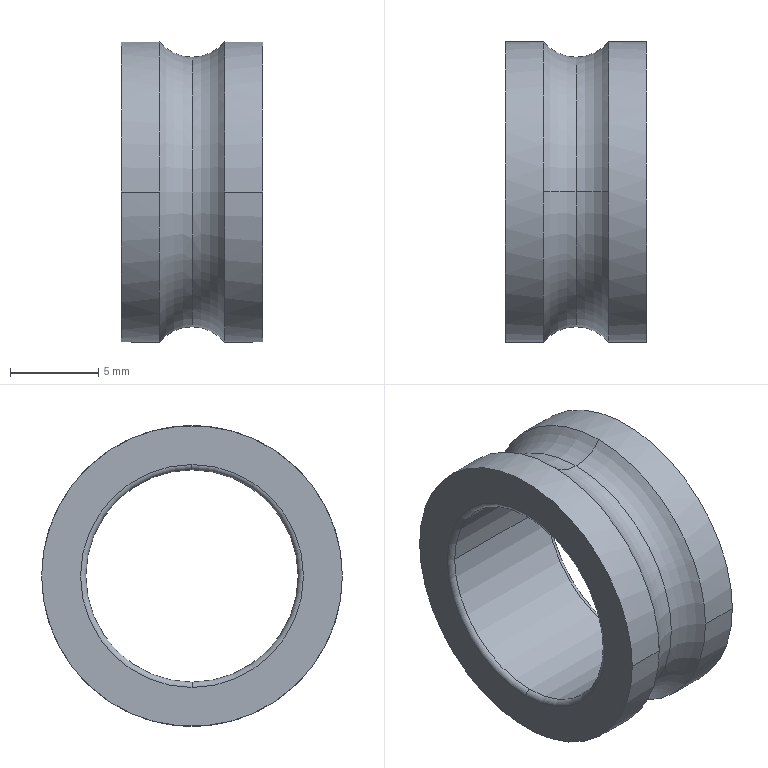Part | STEP file | skf_bearing_6001_2_02 | 1 solid | 16 faces | box 8 x 17 x 17 mm | volume 793.588 mm3 | torus 8 | cylinder 6 | plane 2 | commonest cylinder face diameters 17 x4 12 x2
STEP:
#1=CARTESIAN_POINT('',(5.849,0.,-8.5));
#2=VERTEX_POINT('',#1);
#3=CARTESIAN_POINT('',(4.,0.,-7.619));
#4=VERTEX_POINT('',#3);
#5=CARTESIAN_POINT('',(4.,0.,-10.));
#6=DIRECTION('',(0.,-1.,0.));
#7=DIRECTION('',(0.,0.,-1.));
#8=AXIS2_PLACEMENT_3D('',#5,#6,#7);
#9=CIRCLE('',#8,2.381);
#10=EDGE_CURVE('',#2,#4,#9,.T.);
#11=ORIENTED_EDGE('',*,*,#10,.T.);
#12=CARTESIAN_POINT('',(4.,0.,7.619));
#13=VERTEX_POINT('',#12);
#14=CARTESIAN_POINT('',(4.,0.,0.));
#15=DIRECTION('',(1.,0.,0.));
#16=DIRECTION('',(0.,0.,-1.));
#17=AXIS2_PLACEMENT_3D('',#14,#15,#16);
#18=CIRCLE('',#17,7.619);
#19=EDGE_CURVE('',#4,#13,#18,.T.);
#20=ORIENTED_EDGE('',*,*,#19,.T.);
#21=CARTESIAN_POINT('',(5.849,0.,8.5));
#22=VERTEX_POINT('',#21);
#23=CARTESIAN_POINT('',(4.,0.,10.));
#24=DIRECTION('',(0.,1.,0.));
#25=DIRECTION('',(0.,0.,1.));
#26=AXIS2_PLACEMENT_3D('',#23,#24,#25);
#27=CIRCLE('',#26,2.381);
#28=EDGE_CURVE('',#22,#13,#27,.T.);
#29=ORIENTED_EDGE('',*,*,#28,.F.);
#30=CARTESIAN_POINT('',(5.849,8.5,0.));
#31=VERTEX_POINT('',#30);
#32=CARTESIAN_POINT('',(5.849,0.,0.));
#33=DIRECTION('',(1.,0.,0.));
#34=DIRECTION('',(0.,1.,0.));
#35=AXIS2_PLACEMENT_3D('',#32,#33,#34);
#36=CIRCLE('',#35,8.5);
#37=EDGE_CURVE('',#31,#22,#36,.T.);
#38=ORIENTED_EDGE('',*,*,#37,.F.);
#39=CARTESIAN_POINT('',(5.849,0.,0.));
#40=DIRECTION('',(1.,0.,0.));
#41=DIRECTION('',(0.,1.,0.));
#42=AXIS2_PLACEMENT_3D('',#39,#40,#41);
#43=CIRCLE('',#42,8.5);
#44=EDGE_CURVE('',#2,#31,#43,.T.);
#45=ORIENTED_EDGE('',*,*,#44,.F.);
#46=EDGE_LOOP('',(#11,#20,#29,#38,#45));
#47=FACE_OUTER_BOUND('',#46,.T.);
#48=CARTESIAN_POINT('',(4.,0.,0.));
#49=DIRECTION('',(1.,0.,0.));
#50=DIRECTION('',(0.,0.,-1.));
#51=AXIS2_PLACEMENT_3D('',#48,#49,#50);
#52=TOROIDAL_SURFACE('',#51,10.,2.381);
#53=ADVANCED_FACE('',(#47),#52,.F.);
#54=ORIENTED_EDGE('',*,*,#28,.T.);
#55=CARTESIAN_POINT('',(4.,0.,0.));
#56=DIRECTION('',(1.,0.,0.));
#57=DIRECTION('',(0.,0.,-1.));
#58=AXIS2_PLACEMENT_3D('',#55,#56,#57);
#59=CIRCLE('',#58,7.619);
#60=EDGE_CURVE('',#13,#4,#59,.T.);
#61=ORIENTED_EDGE('',*,*,#60,.T.);
#62=ORIENTED_EDGE('',*,*,#10,.F.);
#63=CARTESIAN_POINT('',(5.849,-8.5,0.));
#64=VERTEX_POINT('',#63);
#65=CARTESIAN_POINT('',(5.849,0.,0.));
#66=DIRECTION('',(1.,0.,0.));
#67=DIRECTION('',(0.,1.,0.));
#68=AXIS2_PLACEMENT_3D('',#65,#66,#67);
#69=CIRCLE('',#68,8.5);
#70=EDGE_CURVE('',#64,#2,#69,.T.);
#71=ORIENTED_EDGE('',*,*,#70,.F.);
#72=CARTESIAN_POINT('',(5.849,0.,0.));
#73=DIRECTION('',(1.,0.,0.));
#74=DIRECTION('',(0.,1.,0.));
#75=AXIS2_PLACEMENT_3D('',#72,#73,#74);
#76=CIRCLE('',#75,8.5);
#77=EDGE_CURVE('',#22,#64,#76,.T.);
#78=ORIENTED_EDGE('',*,*,#77,.F.);
#79=EDGE_LOOP('',(#54,#61,#62,#71,#78));
#80=FACE_OUTER_BOUND('',#79,.T.);
#81=CARTESIAN_POINT('',(4.,0.,0.));
#82=DIRECTION('',(1.,0.,0.));
#83=DIRECTION('',(0.,0.,-1.));
#84=AXIS2_PLACEMENT_3D('',#81,#82,#83);
#85=TOROIDAL_SURFACE('',#84,10.,2.381);
#86=ADVANCED_FACE('',(#80),#85,.F.);
#87=CARTESIAN_POINT('',(8.,0.,-6.3));
#88=VERTEX_POINT('',#87);
#89=CARTESIAN_POINT('',(8.,0.,6.3));
#90=VERTEX_POINT('',#89);
#91=CARTESIAN_POINT('',(8.,0.,0.));
#92=DIRECTION('',(1.,0.,0.));
#93=DIRECTION('',(0.,1.,0.));
#94=AXIS2_PLACEMENT_3D('',#91,#92,#93);
#95=CIRCLE('',#94,6.3);
#96=EDGE_CURVE('',#88,#90,#95,.T.);
#97=ORIENTED_EDGE('',*,*,#96,.T.);
#98=CARTESIAN_POINT('',(7.7,0.,6.));
#99=VERTEX_POINT('',#98);
#100=CARTESIAN_POINT('',(7.7,0.,6.3));
#101=DIRECTION('',(0.,1.,0.));
#102=DIRECTION('',(0.,0.,1.));
#103=AXIS2_PLACEMENT_3D('',#100,#101,#102);
#104=CIRCLE('',#103,0.3);
#105=EDGE_CURVE('',#90,#99,#104,.T.);
#106=ORIENTED_EDGE('',*,*,#105,.T.);
#107=CARTESIAN_POINT('',(7.7,6.,0.));
#108=VERTEX_POINT('',#107);
#109=CARTESIAN_POINT('',(7.7,0.,0.));
#110=DIRECTION('',(1.,0.,0.));
#111=DIRECTION('',(0.,1.,0.));
#112=AXIS2_PLACEMENT_3D('',#109,#110,#111);
#113=CIRCLE('',#112,6.);
#114=EDGE_CURVE('',#108,#99,#113,.T.);
#115=ORIENTED_EDGE('',*,*,#114,.F.);
#116=CARTESIAN_POINT('',(7.7,0.,-6.));
#117=VERTEX_POINT('',#116);
#118=CARTESIAN_POINT('',(7.7,0.,0.));
#119=DIRECTION('',(1.,0.,0.));
#120=DIRECTION('',(0.,1.,0.));
#121=AXIS2_PLACEMENT_3D('',#118,#119,#120);
#122=CIRCLE('',#121,6.);
#123=EDGE_CURVE('',#117,#108,#122,.T.);
#124=ORIENTED_EDGE('',*,*,#123,.F.);
#125=CARTESIAN_POINT('',(7.7,0.,-6.3));
#126=DIRECTION('',(0.,-1.,0.));
#127=DIRECTION('',(0.,0.,-1.));
#128=AXIS2_PLACEMENT_3D('',#125,#126,#127);
#129=CIRCLE('',#128,0.3);
#130=EDGE_CURVE('',#88,#117,#129,.T.);
#131=ORIENTED_EDGE('',*,*,#130,.F.);
#132=EDGE_LOOP('',(#97,#106,#115,#124,#131));
#133=FACE_OUTER_BOUND('',#132,.T.);
#134=CARTESIAN_POINT('',(7.7,0.,0.));
#135=DIRECTION('',(1.,0.,0.));
#136=DIRECTION('',(0.,0.,-1.));
#137=AXIS2_PLACEMENT_3D('',#134,#135,#136);
#138=TOROIDAL_SURFACE('',#137,6.3,0.3);
#139=ADVANCED_FACE('',(#133),#138,.T.);
#140=ORIENTED_EDGE('',*,*,#114,.T.);
#141=CARTESIAN_POINT('',(7.7,-6.,0.));
#142=VERTEX_POINT('',#141);
#143=CARTESIAN_POINT('',(7.7,0.,0.));
#144=DIRECTION('',(1.,0.,0.));
#145=DIRECTION('',(0.,1.,0.));
#146=AXIS2_PLACEMENT_3D('',#143,#144,#145);
#147=CIRCLE('',#146,6.);
#148=EDGE_CURVE('',#99,#142,#147,.T.);
#149=ORIENTED_EDGE('',*,*,#148,.T.);
#150=CARTESIAN_POINT('',(0.3,-6.,0.));
#151=VERTEX_POINT('',#150);
#152=CARTESIAN_POINT('',(4.,-6.,0.));
#153=DIRECTION('',(-1.,0.,0.));
#154=VECTOR('',#153,1000.);
#155=LINE('',#152,#154);
#156=EDGE_CURVE('',#142,#151,#155,.T.);
#157=ORIENTED_EDGE('',*,*,#156,.T.);
#158=CARTESIAN_POINT('',(0.3,0.,6.));
#159=VERTEX_POINT('',#158);
#160=CARTESIAN_POINT('',(0.3,0.,0.));
#161=DIRECTION('',(1.,0.,0.));
#162=DIRECTION('',(0.,1.,0.));
#163=AXIS2_PLACEMENT_3D('',#160,#161,#162);
#164=CIRCLE('',#163,6.);
#165=EDGE_CURVE('',#159,#151,#164,.T.);
#166=ORIENTED_EDGE('',*,*,#165,.F.);
#167=CARTESIAN_POINT('',(0.3,6.,0.));
#168=VERTEX_POINT('',#167);
#169=CARTESIAN_POINT('',(0.3,0.,0.));
#170=DIRECTION('',(1.,0.,0.));
#171=DIRECTION('',(0.,1.,0.));
#172=AXIS2_PLACEMENT_3D('',#169,#170,#171);
#173=CIRCLE('',#172,6.);
#174=EDGE_CURVE('',#168,#159,#173,.T.);
#175=ORIENTED_EDGE('',*,*,#174,.F.);
#176=CARTESIAN_POINT('',(4.,6.,0.));
#177=DIRECTION('',(-1.,0.,0.));
#178=VECTOR('',#177,1000.);
#179=LINE('',#176,#178);
#180=EDGE_CURVE('',#108,#168,#179,.T.);
#181=ORIENTED_EDGE('',*,*,#180,.F.);
#182=EDGE_LOOP('',(#140,#149,#157,#166,#175,#181));
#183=FACE_OUTER_BOUND('',#182,.T.);
#184=CARTESIAN_POINT('',(4.,0.,0.));
#185=DIRECTION('',(-1.,0.,0.));
#186=DIRECTION('',(0.,1.,0.));
#187=AXIS2_PLACEMENT_3D('',#184,#185,#186);
#188=CYLINDRICAL_SURFACE('',#187,6.);
#189=ADVANCED_FACE('',(#183),#188,.F.);
#190=CARTESIAN_POINT('',(0.3,0.,-6.));
#191=VERTEX_POINT('',#190);
#192=CARTESIAN_POINT('',(0.3,0.,0.));
#193=DIRECTION('',(1.,0.,0.));
#194=DIRECTION('',(0.,1.,0.));
#195=AXIS2_PLACEMENT_3D('',#192,#193,#194);
#196=CIRCLE('',#195,6.);
#197=EDGE_CURVE('',#191,#168,#196,.T.);
#198=ORIENTED_EDGE('',*,*,#197,.T.);
#199=ORIENTED_EDGE('',*,*,#174,.T.);
#200=CARTESIAN_POINT('',(0.,0.,6.3));
#201=VERTEX_POINT('',#200);
#202=CARTESIAN_POINT('',(0.3,0.,6.3));
#203=DIRECTION('',(0.,1.,0.));
#204=DIRECTION('',(0.,0.,1.));
#205=AXIS2_PLACEMENT_3D('',#202,#203,#204);
#206=CIRCLE('',#205,0.3);
#207=EDGE_CURVE('',#159,#201,#206,.T.);
#208=ORIENTED_EDGE('',*,*,#207,.T.);
#209=CARTESIAN_POINT('',(0.,0.,-6.3));
#210=VERTEX_POINT('',#209);
#211=CARTESIAN_POINT('',(0.,0.,0.));
#212=DIRECTION('',(1.,0.,0.));
#213=DIRECTION('',(0.,1.,0.));
#214=AXIS2_PLACEMENT_3D('',#211,#212,#213);
#215=CIRCLE('',#214,6.3);
#216=EDGE_CURVE('',#210,#201,#215,.T.);
#217=ORIENTED_EDGE('',*,*,#216,.F.);
#218=CARTESIAN_POINT('',(0.3,0.,-6.3));
#219=DIRECTION('',(0.,-1.,0.));
#220=DIRECTION('',(0.,0.,-1.));
#221=AXIS2_PLACEMENT_3D('',#218,#219,#220);
#222=CIRCLE('',#221,0.3);
#223=EDGE_CURVE('',#191,#210,#222,.T.);
#224=ORIENTED_EDGE('',*,*,#223,.F.);
#225=EDGE_LOOP('',(#198,#199,#208,#217,#224));
#226=FACE_OUTER_BOUND('',#225,.T.);
#227=CARTESIAN_POINT('',(0.3,0.,0.));
#228=DIRECTION('',(1.,0.,0.));
#229=DIRECTION('',(0.,0.,-1.));
#230=AXIS2_PLACEMENT_3D('',#227,#228,#229);
#231=TOROIDAL_SURFACE('',#230,6.3,0.3);
#232=ADVANCED_FACE('',(#226),#231,.T.);
#233=CARTESIAN_POINT('',(2.151,-8.5,0.));
#234=VERTEX_POINT('',#233);
#235=CARTESIAN_POINT('',(2.151,0.,-8.5));
#236=VERTEX_POINT('',#235);
#237=CARTESIAN_POINT('',(2.151,0.,0.));
#238=DIRECTION('',(1.,0.,0.));
#239=DIRECTION('',(0.,1.,0.));
#240=AXIS2_PLACEMENT_3D('',#237,#238,#239);
#241=CIRCLE('',#240,8.5);
#242=EDGE_CURVE('',#234,#236,#241,.T.);
#243=ORIENTED_EDGE('',*,*,#242,.F.);
#244=CARTESIAN_POINT('',(0.,-8.5,0.));
#245=VERTEX_POINT('',#244);
#246=CARTESIAN_POINT('',(1.075,-8.5,0.));
#247=DIRECTION('',(-1.,0.,0.));
#248=VECTOR('',#247,1000.);
#249=LINE('',#246,#248);
#250=EDGE_CURVE('',#234,#245,#249,.T.);
#251=ORIENTED_EDGE('',*,*,#250,.T.);
#252=CARTESIAN_POINT('',(0.,8.5,0.));
#253=VERTEX_POINT('',#252);
#254=CARTESIAN_POINT('',(0.,0.,0.));
#255=DIRECTION('',(1.,0.,0.));
#256=DIRECTION('',(0.,1.,0.));
#257=AXIS2_PLACEMENT_3D('',#254,#255,#256);
#258=CIRCLE('',#257,8.5);
#259=EDGE_CURVE('',#245,#253,#258,.T.);
#260=ORIENTED_EDGE('',*,*,#259,.T.);
#261=CARTESIAN_POINT('',(2.151,8.5,0.));
#262=VERTEX_POINT('',#261);
#263=CARTESIAN_POINT('',(1.075,8.5,0.));
#264=DIRECTION('',(-1.,0.,0.));
#265=VECTOR('',#264,1000.);
#266=LINE('',#263,#265);
#267=EDGE_CURVE('',#262,#253,#266,.T.);
#268=ORIENTED_EDGE('',*,*,#267,.F.);
#269=CARTESIAN_POINT('',(2.151,0.,0.));
#270=DIRECTION('',(1.,0.,0.));
#271=DIRECTION('',(0.,1.,0.));
#272=AXIS2_PLACEMENT_3D('',#269,#270,#271);
#273=CIRCLE('',#272,8.5);
#274=EDGE_CURVE('',#236,#262,#273,.T.);
#275=ORIENTED_EDGE('',*,*,#274,.F.);
#276=EDGE_LOOP('',(#243,#251,#260,#268,#275));
#277=FACE_OUTER_BOUND('',#276,.T.);
#278=CARTESIAN_POINT('',(1.075,0.,0.));
#279=DIRECTION('',(-1.,0.,0.));
#280=DIRECTION('',(0.,1.,0.));
#281=AXIS2_PLACEMENT_3D('',#278,#279,#280);
#282=CYLINDRICAL_SURFACE('',#281,8.5);
#283=ADVANCED_FACE('',(#277),#282,.T.);
#284=ORIENTED_EDGE('',*,*,#60,.F.);
#285=CARTESIAN_POINT('',(2.151,0.,8.5));
#286=VERTEX_POINT('',#285);
#287=CARTESIAN_POINT('',(4.,0.,10.));
#288=DIRECTION('',(0.,1.,0.));
#289=DIRECTION('',(0.,0.,1.));
#290=AXIS2_PLACEMENT_3D('',#287,#288,#289);
#291=CIRCLE('',#290,2.381);
#292=EDGE_CURVE('',#13,#286,#291,.T.);
#293=ORIENTED_EDGE('',*,*,#292,.T.);
#294=CARTESIAN_POINT('',(2.151,0.,0.));
#295=DIRECTION('',(1.,0.,0.));
#296=DIRECTION('',(0.,1.,0.));
#297=AXIS2_PLACEMENT_3D('',#294,#295,#296);
#298=CIRCLE('',#297,8.5);
#299=EDGE_CURVE('',#286,#234,#298,.T.);
#300=ORIENTED_EDGE('',*,*,#299,.T.);
#301=ORIENTED_EDGE('',*,*,#242,.T.);
#302=CARTESIAN_POINT('',(4.,0.,-10.));
#303=DIRECTION('',(0.,-1.,0.));
#304=DIRECTION('',(0.,0.,-1.));
#305=AXIS2_PLACEMENT_3D('',#302,#303,#304);
#306=CIRCLE('',#305,2.381);
#307=EDGE_CURVE('',#4,#236,#306,.T.);
#308=ORIENTED_EDGE('',*,*,#307,.F.);
#309=EDGE_LOOP('',(#284,#293,#300,#301,#308));
#310=FACE_OUTER_BOUND('',#309,.T.);
#311=CARTESIAN_POINT('',(4.,0.,0.));
#312=DIRECTION('',(1.,0.,0.));
#313=DIRECTION('',(0.,0.,-1.));
#314=AXIS2_PLACEMENT_3D('',#311,#312,#313);
#315=TOROIDAL_SURFACE('',#314,10.,2.381);
#316=ADVANCED_FACE('',(#310),#315,.F.);
#317=CARTESIAN_POINT('',(8.,-8.5,0.));
#318=VERTEX_POINT('',#317);
#319=CARTESIAN_POINT('',(8.,8.5,0.));
#320=VERTEX_POINT('',#319);
#321=CARTESIAN_POINT('',(8.,0.,0.));
#322=DIRECTION('',(1.,0.,0.));
#323=DIRECTION('',(0.,1.,0.));
#324=AXIS2_PLACEMENT_3D('',#321,#322,#323);
#325=CIRCLE('',#324,8.5);
#326=EDGE_CURVE('',#318,#320,#325,.T.);
#327=ORIENTED_EDGE('',*,*,#326,.F.);
#328=CARTESIAN_POINT('',(6.925,-8.5,0.));
#329=DIRECTION('',(-1.,0.,0.));
#330=VECTOR('',#329,1000.);
#331=LINE('',#328,#330);
#332=EDGE_CURVE('',#318,#64,#331,.T.);
#333=ORIENTED_EDGE('',*,*,#332,.T.);
#334=ORIENTED_EDGE('',*,*,#70,.T.);
#335=ORIENTED_EDGE('',*,*,#44,.T.);
#336=CARTESIAN_POINT('',(6.925,8.5,0.));
#337=DIRECTION('',(-1.,0.,0.));
#338=VECTOR('',#337,1000.);
#339=LINE('',#336,#338);
#340=EDGE_CURVE('',#320,#31,#339,.T.);
#341=ORIENTED_EDGE('',*,*,#340,.F.);
#342=EDGE_LOOP('',(#327,#333,#334,#335,#341));
#343=FACE_OUTER_BOUND('',#342,.T.);
#344=CARTESIAN_POINT('',(6.925,0.,0.));
#345=DIRECTION('',(-1.,0.,0.));
#346=DIRECTION('',(0.,1.,0.));
#347=AXIS2_PLACEMENT_3D('',#344,#345,#346);
#348=CYLINDRICAL_SURFACE('',#347,8.5);
#349=ADVANCED_FACE('',(#343),#348,.T.);
#350=ORIENTED_EDGE('',*,*,#332,.F.);
#351=CARTESIAN_POINT('',(8.,0.,0.));
#352=DIRECTION('',(1.,0.,0.));
#353=DIRECTION('',(0.,1.,0.));
#354=AXIS2_PLACEMENT_3D('',#351,#352,#353);
#355=CIRCLE('',#354,8.5);
#356=EDGE_CURVE('',#320,#318,#355,.T.);
#357=ORIENTED_EDGE('',*,*,#356,.F.);
#358=ORIENTED_EDGE('',*,*,#340,.T.);
#359=ORIENTED_EDGE('',*,*,#37,.T.);
#360=ORIENTED_EDGE('',*,*,#77,.T.);
#361=EDGE_LOOP('',(#350,#357,#358,#359,#360));
#362=FACE_OUTER_BOUND('',#361,.T.);
#363=CARTESIAN_POINT('',(6.925,0.,0.));
#364=DIRECTION('',(-1.,0.,0.));
#365=DIRECTION('',(0.,1.,0.));
#366=AXIS2_PLACEMENT_3D('',#363,#364,#365);
#367=CYLINDRICAL_SURFACE('',#366,8.5);
#368=ADVANCED_FACE('',(#362),#367,.T.);
#369=ORIENTED_EDGE('',*,*,#19,.F.);
#370=ORIENTED_EDGE('',*,*,#307,.T.);
#371=ORIENTED_EDGE('',*,*,#274,.T.);
#372=CARTESIAN_POINT('',(2.151,0.,0.));
#373=DIRECTION('',(1.,0.,0.));
#374=DIRECTION('',(0.,1.,0.));
#375=AXIS2_PLACEMENT_3D('',#372,#373,#374);
#376=CIRCLE('',#375,8.5);
#377=EDGE_CURVE('',#262,#286,#376,.T.);
#378=ORIENTED_EDGE('',*,*,#377,.T.);
#379=ORIENTED_EDGE('',*,*,#292,.F.);
#380=EDGE_LOOP('',(#369,#370,#371,#378,#379));
#381=FACE_OUTER_BOUND('',#380,.T.);
#382=CARTESIAN_POINT('',(4.,0.,0.));
#383=DIRECTION('',(1.,0.,0.));
#384=DIRECTION('',(0.,0.,-1.));
#385=AXIS2_PLACEMENT_3D('',#382,#383,#384);
#386=TOROIDAL_SURFACE('',#385,10.,2.381);
#387=ADVANCED_FACE('',(#381),#386,.F.);
#388=ORIENTED_EDGE('',*,*,#250,.F.);
#389=ORIENTED_EDGE('',*,*,#299,.F.);
#390=ORIENTED_EDGE('',*,*,#377,.F.);
#391=ORIENTED_EDGE('',*,*,#267,.T.);
#392=CARTESIAN_POINT('',(0.,0.,0.));
#393=DIRECTION('',(1.,0.,0.));
#394=DIRECTION('',(0.,1.,0.));
#395=AXIS2_PLACEMENT_3D('',#392,#393,#394);
#396=CIRCLE('',#395,8.5);
#397=EDGE_CURVE('',#253,#245,#396,.T.);
#398=ORIENTED_EDGE('',*,*,#397,.T.);
#399=EDGE_LOOP('',(#388,#389,#390,#391,#398));
#400=FACE_OUTER_BOUND('',#399,.T.);
#401=CARTESIAN_POINT('',(1.075,0.,0.));
#402=DIRECTION('',(-1.,0.,0.));
#403=DIRECTION('',(0.,1.,0.));
#404=AXIS2_PLACEMENT_3D('',#401,#402,#403);
#405=CYLINDRICAL_SURFACE('',#404,8.5);
#406=ADVANCED_FACE('',(#400),#405,.T.);
#407=ORIENTED_EDGE('',*,*,#216,.T.);
#408=CARTESIAN_POINT('',(0.,0.,0.));
#409=DIRECTION('',(1.,0.,0.));
#410=DIRECTION('',(0.,1.,0.));
#411=AXIS2_PLACEMENT_3D('',#408,#409,#410);
#412=CIRCLE('',#411,6.3);
#413=EDGE_CURVE('',#201,#210,#412,.T.);
#414=ORIENTED_EDGE('',*,*,#413,.T.);
#415=EDGE_LOOP('',(#407,#414));
#416=FACE_BOUND('',#415,.T.);
#417=ORIENTED_EDGE('',*,*,#397,.F.);
#418=ORIENTED_EDGE('',*,*,#259,.F.);
#419=EDGE_LOOP('',(#417,#418));
#420=FACE_OUTER_BOUND('',#419,.T.);
#421=CARTESIAN_POINT('',(0.,7.4,0.));
#422=DIRECTION('',(-1.,0.,0.));
#423=DIRECTION('',(0.,-1.,0.));
#424=AXIS2_PLACEMENT_3D('',#421,#422,#423);
#425=PLANE('',#424);
#426=ADVANCED_FACE('',(#416,#420),#425,.T.);
#427=ORIENTED_EDGE('',*,*,#207,.F.);
#428=ORIENTED_EDGE('',*,*,#165,.T.);
#429=CARTESIAN_POINT('',(0.3,0.,0.));
#430=DIRECTION('',(1.,0.,0.));
#431=DIRECTION('',(0.,1.,0.));
#432=AXIS2_PLACEMENT_3D('',#429,#430,#431);
#433=CIRCLE('',#432,6.);
#434=EDGE_CURVE('',#151,#191,#433,.T.);
#435=ORIENTED_EDGE('',*,*,#434,.T.);
#436=ORIENTED_EDGE('',*,*,#223,.T.);
#437=ORIENTED_EDGE('',*,*,#413,.F.);
#438=EDGE_LOOP('',(#427,#428,#435,#436,#437));
#439=FACE_OUTER_BOUND('',#438,.T.);
#440=CARTESIAN_POINT('',(0.3,0.,0.));
#441=DIRECTION('',(1.,0.,0.));
#442=DIRECTION('',(0.,0.,-1.));
#443=AXIS2_PLACEMENT_3D('',#440,#441,#442);
#444=TOROIDAL_SURFACE('',#443,6.3,0.3);
#445=ADVANCED_FACE('',(#439),#444,.T.);
#446=ORIENTED_EDGE('',*,*,#156,.F.);
#447=CARTESIAN_POINT('',(7.7,0.,0.));
#448=DIRECTION('',(1.,0.,0.));
#449=DIRECTION('',(0.,1.,0.));
#450=AXIS2_PLACEMENT_3D('',#447,#448,#449);
#451=CIRCLE('',#450,6.);
#452=EDGE_CURVE('',#142,#117,#451,.T.);
#453=ORIENTED_EDGE('',*,*,#452,.T.);
#454=ORIENTED_EDGE('',*,*,#123,.T.);
#455=ORIENTED_EDGE('',*,*,#180,.T.);
#456=ORIENTED_EDGE('',*,*,#197,.F.);
#457=ORIENTED_EDGE('',*,*,#434,.F.);
#458=EDGE_LOOP('',(#446,#453,#454,#455,#456,#457));
#459=FACE_OUTER_BOUND('',#458,.T.);
#460=CARTESIAN_POINT('',(4.,0.,0.));
#461=DIRECTION('',(-1.,0.,0.));
#462=DIRECTION('',(0.,1.,0.));
#463=AXIS2_PLACEMENT_3D('',#460,#461,#462);
#464=CYLINDRICAL_SURFACE('',#463,6.);
#465=ADVANCED_FACE('',(#459),#464,.F.);
#466=ORIENTED_EDGE('',*,*,#105,.F.);
#467=CARTESIAN_POINT('',(8.,0.,0.));
#468=DIRECTION('',(1.,0.,0.));
#469=DIRECTION('',(0.,1.,0.));
#470=AXIS2_PLACEMENT_3D('',#467,#468,#469);
#471=CIRCLE('',#470,6.3);
#472=EDGE_CURVE('',#90,#88,#471,.T.);
#473=ORIENTED_EDGE('',*,*,#472,.T.);
#474=ORIENTED_EDGE('',*,*,#130,.T.);
#475=ORIENTED_EDGE('',*,*,#452,.F.);
#476=ORIENTED_EDGE('',*,*,#148,.F.);
#477=EDGE_LOOP('',(#466,#473,#474,#475,#476));
#478=FACE_OUTER_BOUND('',#477,.T.);
#479=CARTESIAN_POINT('',(7.7,0.,0.));
#480=DIRECTION('',(1.,0.,0.));
#481=DIRECTION('',(0.,0.,-1.));
#482=AXIS2_PLACEMENT_3D('',#479,#480,#481);
#483=TOROIDAL_SURFACE('',#482,6.3,0.3);
#484=ADVANCED_FACE('',(#478),#483,.T.);
#485=ORIENTED_EDGE('',*,*,#356,.T.);
#486=ORIENTED_EDGE('',*,*,#326,.T.);
#487=EDGE_LOOP('',(#485,#486));
#488=FACE_OUTER_BOUND('',#487,.T.);
#489=ORIENTED_EDGE('',*,*,#96,.F.);
#490=ORIENTED_EDGE('',*,*,#472,.F.);
#491=EDGE_LOOP('',(#489,#490));
#492=FACE_BOUND('',#491,.T.);
#493=CARTESIAN_POINT('',(8.,7.4,0.));
#494=DIRECTION('',(1.,0.,0.));
#495=DIRECTION('',(0.,1.,0.));
#496=AXIS2_PLACEMENT_3D('',#493,#494,#495);
#497=PLANE('',#496);
#498=ADVANCED_FACE('',(#488,#492),#497,.T.);
#499=CLOSED_SHELL('',(#53,#86,#139,#189,#232,#283,#316,#349,#368,#387,#406,#426,#445,#465,#484,#498));
#500=MANIFOLD_SOLID_BREP('',#499);
#501=CARTESIAN_POINT('',(0.,0.,0.));
#502=DIRECTION('',(0.,0.,1.));
#503=DIRECTION('',(1.,0.,0.));
#504=AXIS2_PLACEMENT_3D('',#501,#502,#503);
#505=(LENGTH_UNIT()NAMED_UNIT(*)SI_UNIT(.MILLI.,.METRE.));
#506=UNCERTAINTY_MEASURE_WITH_UNIT(LENGTH_MEASURE(0.00001),#505,'','');
#507=(NAMED_UNIT(*)PLANE_ANGLE_UNIT()SI_UNIT($,.RADIAN.));
#508=(NAMED_UNIT(*)SI_UNIT($,.STERADIAN.)SOLID_ANGLE_UNIT());
#509=(GEOMETRIC_REPRESENTATION_CONTEXT(3)GLOBAL_UNCERTAINTY_ASSIGNED_CONTEXT((#506))GLOBAL_UNIT_ASSIGNED_CONTEXT((#505,#507,#508))REPRESENTATION_CONTEXT('',''));
#510=ADVANCED_BREP_SHAPE_REPRESENTATION('',(#500,#504),#509);